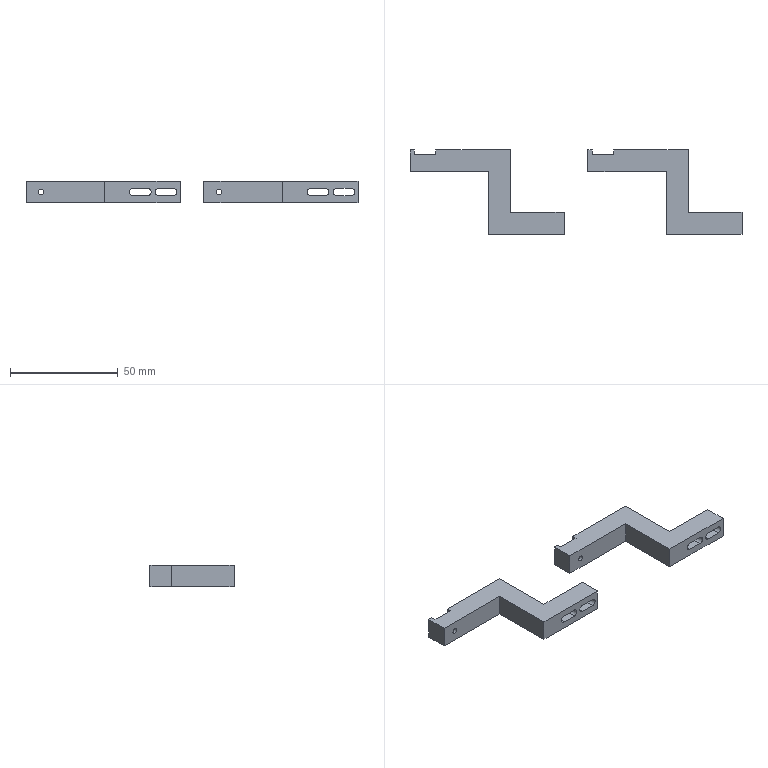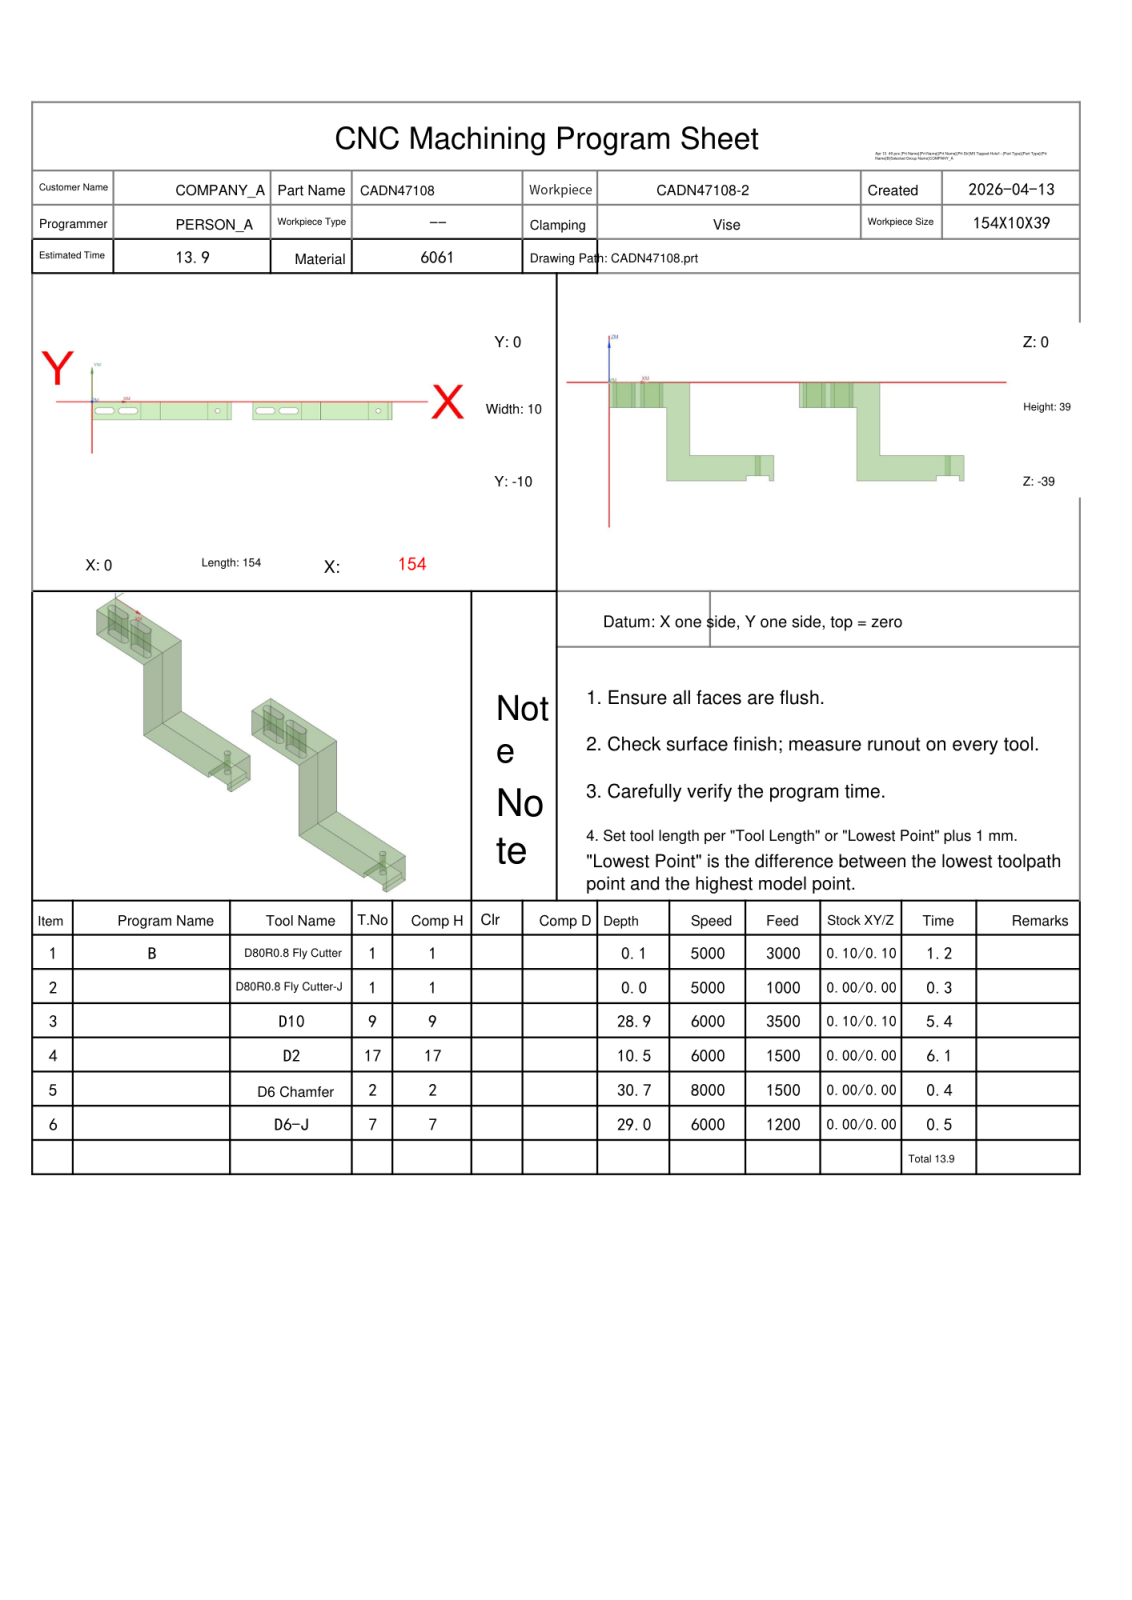NC program | NX | posted by the shop | part box 154 x 39 x 10 mm
Lines 2223 to 3149 of 5887:
N4 T17 M06
(D2  D=2. R=0. H=17 ce=0.10 di=0.10)
G00 G90 G54 X18.5 Y-4.4 M03 S6000
G43 H17 Z20.
M08
Z.5
G01 X15.2 Z.481 F1500.
G03 X14.6 Y-5. Z.475 I0.0 J-.6
X15.2 Y-5.6 Z.47 I.6 J0.0
G01 X21.8 Z.431
G03 X22.4 Y-5. Z.426 I0.0 J.6
X21.8 Y-4.4 Z.42 I-.6 J0.0
G01 X15.2 Z.382
G03 X14.6 Y-5. Z.376 I0.0 J-.6
X15.2 Y-5.6 Z.371 I.6 J0.0
G01 X21.8 Z.332
G03 X22.4 Y-5. Z.327 I0.0 J.6
X21.8 Y-4.4 Z.321 I-.6 J0.0
G01 X15.2 Z.283
G03 X14.6 Y-5. Z.277 I0.0 J-.6
X15.2 Y-5.6 Z.272 I.6 J0.0
G01 X21.8 Z.233
G03 X22.4 Y-5. Z.227 I0.0 J.6
X21.8 Y-4.4 Z.222 I-.6 J0.0
G01 X15.2 Z.183
G03 X14.6 Y-5. Z.178 I0.0 J-.6
X15.2 Y-5.6 Z.172 I.6 J0.0
G01 X21.8 Z.134
G03 X22.4 Y-5. Z.128 I0.0 J.6
X21.8 Y-4.4 Z.123 I-.6 J0.0
G01 X15.2 Z.084
G03 X14.6 Y-5. Z.079 I0.0 J-.6
X15.2 Y-5.6 Z.073 I.6 J0.0
G01 X21.8 Z.035
G03 X22.4 Y-5. Z.029 I0.0 J.6
X21.8 Y-4.4 Z.024 I-.6 J0.0
G01 X15.2 Z-.015
G03 X14.6 Y-5. Z-.02 I0.0 J-.6
X15.2 Y-5.6 Z-.026 I.6 J0.0
G01 X21.8 Z-.064
G03 X22.4 Y-5. Z-.07 I0.0 J.6
X21.8 Y-4.4 Z-.075 I-.6 J0.0
G01 X15.2 Z-.114
G03 X14.6 Y-5. Z-.119 I0.0 J-.6
X15.2 Y-5.6 Z-.125 I.6 J0.0
G01 X21.8 Z-.163
G03 X22.4 Y-5. Z-.169 I0.0 J.6
X21.8 Y-4.4 Z-.174 I-.6 J0.0
G01 X15.2 Z-.213
G03 X14.6 Y-5. Z-.218 I0.0 J-.6
X15.2 Y-5.6 Z-.224 I.6 J0.0
G01 X21.8 Z-.263
G03 X22.4 Y-5. Z-.268 I0.0 J.6
X21.8 Y-4.4 Z-.274 I-.6 J0.0
G01 X15.2 Z-.312
G03 X14.6 Y-5. Z-.318 I0.0 J-.6
X15.2 Y-5.6 Z-.323 I.6 J0.0
G01 X21.8 Z-.362
G03 X22.4 Y-5. Z-.367 I0.0 J.6
X21.8 Y-4.4 Z-.373 I-.6 J0.0
G01 X15.2 Z-.411
G03 X14.6 Y-5. Z-.417 I0.0 J-.6
X15.2 Y-5.6 Z-.422 I.6 J0.0
G01 X21.8 Z-.461
G03 X22.4 Y-5. Z-.466 I0.0 J.6
X21.8 Y-4.4 Z-.472 I-.6 J0.0
G01 X15.2 Z-.51
G03 X14.6 Y-5. Z-.516 I0.0 J-.6
X15.2 Y-5.6 Z-.521 I.6 J0.0
G01 X21.8 Z-.56
G03 X22.4 Y-5. Z-.565 I0.0 J.6
X21.8 Y-4.4 Z-.571 I-.6 J0.0
G01 X15.2 Z-.609
G03 X14.6 Y-5. Z-.615 I0.0 J-.6
X15.2 Y-5.6 Z-.62 I.6 J0.0
G01 X21.8 Z-.659
G03 X22.4 Y-5. Z-.664 I0.0 J.6
X21.8 Y-4.4 Z-.67 I-.6 J0.0
G01 X15.2 Z-.708
G03 X14.6 Y-5. Z-.714 I0.0 J-.6
X15.2 Y-5.6 Z-.719 I.6 J0.0
G01 X21.8 Z-.758
G03 X22.4 Y-5. Z-.764 I0.0 J.6
X21.8 Y-4.4 Z-.769 I-.6 J0.0
G01 X15.2 Z-.808
G03 X14.6 Y-5. Z-.813 I0.0 J-.6
X15.2 Y-5.6 Z-.819 I.6 J0.0
G01 X21.8 Z-.857
G03 X22.4 Y-5. Z-.863 I0.0 J.6
X21.8 Y-4.4 Z-.868 I-.6 J0.0
G01 X15.2 Z-.907
G03 X14.6 Y-5. Z-.912 I0.0 J-.6
X15.2 Y-5.6 Z-.918 I.6 J0.0
G01 X21.8 Z-.956
G03 X22.4 Y-5. Z-.962 I0.0 J.6
X21.8 Y-4.4 Z-.967 I-.6 J0.0
G01 X15.2 Z-1.006
G03 X14.6 Y-5. Z-1.011 I0.0 J-.6
X15.2 Y-5.6 Z-1.017 I.6 J0.0
G01 X21.8 Z-1.055
G03 X22.4 Y-5. Z-1.061 I0.0 J.6
X21.8 Y-4.4 Z-1.066 I-.6 J0.0
G01 X15.2 Z-1.105
G03 X14.6 Y-5. Z-1.11 I0.0 J-.6
X15.2 Y-5.6 Z-1.116 I.6 J0.0
G01 X21.8 Z-1.154
G03 X22.4 Y-5. Z-1.16 I0.0 J.6
X21.8 Y-4.4 Z-1.165 I-.6 J0.0
G01 X15.2 Z-1.204
G03 X14.6 Y-5. Z-1.209 I0.0 J-.6
X15.2 Y-5.6 Z-1.215 I.6 J0.0
G01 X21.8 Z-1.254
G03 X22.4 Y-5. Z-1.259 I0.0 J.6
X21.8 Y-4.4 Z-1.265 I-.6 J0.0
G01 X15.2 Z-1.303
G03 X14.6 Y-5. Z-1.309 I0.0 J-.6
X15.2 Y-5.6 Z-1.314 I.6 J0.0
G01 X21.8 Z-1.353
G03 X22.4 Y-5. Z-1.358 I0.0 J.6
X21.8 Y-4.4 Z-1.364 I-.6 J0.0
G01 X15.2 Z-1.402
G03 X14.6 Y-5. Z-1.408 I0.0 J-.6
X15.2 Y-5.6 Z-1.413 I.6 J0.0
G01 X21.8 Z-1.452
G03 X22.4 Y-5. Z-1.457 I0.0 J.6
X21.8 Y-4.4 Z-1.463 I-.6 J0.0
G01 X15.2 Z-1.501
G03 X14.6 Y-5. Z-1.507 I0.0 J-.6
X15.2 Y-5.6 Z-1.512 I.6 J0.0
G01 X21.8 Z-1.551
G03 X22.4 Y-5. Z-1.556 I0.0 J.6
X21.8 Y-4.4 Z-1.562 I-.6 J0.0
G01 X15.2 Z-1.6
G03 X14.6 Y-5. Z-1.606 I0.0 J-.6
X15.2 Y-5.6 Z-1.611 I.6 J0.0
G01 X21.8 Z-1.65
G03 X22.4 Y-5. Z-1.655 I0.0 J.6
X21.8 Y-4.4 Z-1.661 I-.6 J0.0
G01 X15.2 Z-1.699
G03 X14.6 Y-5. Z-1.705 I0.0 J-.6
X15.2 Y-5.6 Z-1.71 I.6 J0.0
G01 X21.8 Z-1.749
G03 X22.4 Y-5. Z-1.755 I0.0 J.6
X21.8 Y-4.4 Z-1.76 I-.6 J0.0
G01 X15.2 Z-1.799
G03 X14.6 Y-5. Z-1.804 I0.0 J-.6
X15.2 Y-5.6 Z-1.81 I.6 J0.0
G01 X21.8 Z-1.848
G03 X22.4 Y-5. Z-1.854 I0.0 J.6
X21.8 Y-4.4 Z-1.859 I-.6 J0.0
G01 X15.2 Z-1.898
G03 X14.6 Y-5. Z-1.903 I0.0 J-.6
X15.2 Y-5.6 Z-1.909 I.6 J0.0
G01 X21.8 Z-1.947
G03 X22.4 Y-5. Z-1.953 I0.0 J.6
X21.8 Y-4.4 Z-1.958 I-.6 J0.0
G01 X15.2 Z-1.997
G03 X14.6 Y-5. Z-2.002 I0.0 J-.6
X15.2 Y-5.6 Z-2.008 I.6 J0.0
G01 X21.8 Z-2.046
G03 X22.4 Y-5. Z-2.052 I0.0 J.6
X21.8 Y-4.4 Z-2.057 I-.6 J0.0
G01 X15.2 Z-2.096
G03 X14.6 Y-5. Z-2.101 I0.0 J-.6
X15.2 Y-5.6 Z-2.107 I.6 J0.0
G01 X21.8 Z-2.145
G03 X22.4 Y-5. Z-2.151 I0.0 J.6
X21.8 Y-4.4 Z-2.156 I-.6 J0.0
G01 X15.2 Z-2.195
G03 X14.6 Y-5. Z-2.2 I0.0 J-.6
X15.2 Y-5.6 Z-2.206 I.6 J0.0
G01 X21.8 Z-2.244
G03 X22.4 Y-5. Z-2.25 I0.0 J.6
X21.8 Y-4.4 Z-2.256 I-.6 J0.0
G01 X15.2 Z-2.294
G03 X14.6 Y-5. Z-2.3 I0.0 J-.6
X15.2 Y-5.6 Z-2.305 I.6 J0.0
G01 X21.8 Z-2.344
G03 X22.4 Y-5. Z-2.349 I0.0 J.6
X21.8 Y-4.4 Z-2.355 I-.6 J0.0
G01 X15.2 Z-2.393
G03 X14.6 Y-5. Z-2.399 I0.0 J-.6
X15.2 Y-5.6 Z-2.404 I.6 J0.0
G01 X21.8 Z-2.443
G03 X22.4 Y-5. Z-2.448 I0.0 J.6
X21.8 Y-4.4 Z-2.454 I-.6 J0.0
G01 X15.2 Z-2.492
G03 X14.6 Y-5. Z-2.498 I0.0 J-.6
X15.2 Y-5.6 Z-2.503 I.6 J0.0
G01 X21.8 Z-2.542
G03 X22.4 Y-5. Z-2.547 I0.0 J.6
X21.8 Y-4.4 Z-2.553 I-.6 J0.0
G01 X15.2 Z-2.591
G03 X14.6 Y-5. Z-2.597 I0.0 J-.6
X15.2 Y-5.6 Z-2.602 I.6 J0.0
G01 X21.8 Z-2.641
G03 X22.4 Y-5. Z-2.646 I0.0 J.6
X21.8 Y-4.4 Z-2.652 I-.6 J0.0
G01 X15.2 Z-2.69
G03 X14.6 Y-5. Z-2.696 I0.0 J-.6
X15.2 Y-5.6 Z-2.701 I.6 J0.0
G01 X21.8 Z-2.74
G03 X22.4 Y-5. Z-2.745 I0.0 J.6
X21.8 Y-4.4 Z-2.751 I-.6 J0.0
G01 X15.2 Z-2.79
G03 X14.6 Y-5. Z-2.795 I0.0 J-.6
X15.2 Y-5.6 Z-2.801 I.6 J0.0
G01 X21.8 Z-2.839
G03 X22.4 Y-5. Z-2.845 I0.0 J.6
X21.8 Y-4.4 Z-2.85 I-.6 J0.0
G01 X15.2 Z-2.889
G03 X14.6 Y-5. Z-2.894 I0.0 J-.6
X15.2 Y-5.6 Z-2.9 I.6 J0.0
G01 X21.8 Z-2.938
G03 X22.4 Y-5. Z-2.944 I0.0 J.6
X21.8 Y-4.4 Z-2.949 I-.6 J0.0
G01 X15.2 Z-2.988
G03 X14.6 Y-5. Z-2.993 I0.0 J-.6
X15.2 Y-5.6 Z-2.999 I.6 J0.0
G01 X21.8 Z-3.037
G03 X22.4 Y-5. Z-3.043 I0.0 J.6
X21.8 Y-4.4 Z-3.048 I-.6 J0.0
G01 X15.2 Z-3.087
G03 X14.6 Y-5. Z-3.092 I0.0 J-.6
X15.2 Y-5.6 Z-3.098 I.6 J0.0
G01 X21.8 Z-3.136
G03 X22.4 Y-5. Z-3.142 I0.0 J.6
X21.8 Y-4.4 Z-3.147 I-.6 J0.0
G01 X15.2 Z-3.186
G03 X14.6 Y-5. Z-3.191 I0.0 J-.6
X15.2 Y-5.6 Z-3.197 I.6 J0.0
G01 X21.8 Z-3.235
G03 X22.4 Y-5. Z-3.241 I0.0 J.6
X21.8 Y-4.4 Z-3.246 I-.6 J0.0
G01 X15.2 Z-3.285
G03 X14.6 Y-5. Z-3.291 I0.0 J-.6
X15.2 Y-5.6 Z-3.296 I.6 J0.0
G01 X21.8 Z-3.335
G03 X22.4 Y-5. Z-3.34 I0.0 J.6
X21.8 Y-4.4 Z-3.346 I-.6 J0.0
G01 X15.2 Z-3.384
G03 X14.6 Y-5. Z-3.39 I0.0 J-.6
X15.2 Y-5.6 Z-3.395 I.6 J0.0
G01 X21.8 Z-3.434
G03 X22.4 Y-5. Z-3.439 I0.0 J.6
X21.8 Y-4.4 Z-3.445 I-.6 J0.0
G01 X15.2 Z-3.483
G03 X14.6 Y-5. Z-3.489 I0.0 J-.6
X15.2 Y-5.6 Z-3.494 I.6 J0.0
G01 X21.8 Z-3.533
G03 X22.4 Y-5. Z-3.538 I0.0 J.6
X21.8 Y-4.4 Z-3.544 I-.6 J0.0
G01 X15.2 Z-3.582
G03 X14.6 Y-5. Z-3.588 I0.0 J-.6
X15.2 Y-5.6 Z-3.593 I.6 J0.0
G01 X21.8 Z-3.632
G03 X22.4 Y-5. Z-3.637 I0.0 J.6
X21.8 Y-4.4 Z-3.643 I-.6 J0.0
G01 X15.2 Z-3.681
G03 X14.6 Y-5. Z-3.687 I0.0 J-.6
X15.2 Y-5.6 Z-3.692 I.6 J0.0
G01 X21.8 Z-3.731
G03 X22.4 Y-5. Z-3.736 I0.0 J.6
X21.8 Y-4.4 Z-3.742 I-.6 J0.0
G01 X15.2 Z-3.781
G03 X14.6 Y-5. Z-3.786 I0.0 J-.6
X15.2 Y-5.6 Z-3.792 I.6 J0.0
G01 X21.8 Z-3.83
G03 X22.4 Y-5. Z-3.836 I0.0 J.6
X21.8 Y-4.4 Z-3.841 I-.6 J0.0
G01 X15.2 Z-3.88
G03 X14.6 Y-5. Z-3.885 I0.0 J-.6
X15.2 Y-5.6 Z-3.891 I.6 J0.0
G01 X21.8 Z-3.929
G03 X22.4 Y-5. Z-3.935 I0.0 J.6
X21.8 Y-4.4 Z-3.94 I-.6 J0.0
G01 X15.2 Z-3.979
G03 X14.6 Y-5. Z-3.984 I0.0 J-.6
X15.2 Y-5.6 Z-3.99 I.6 J0.0
G01 X21.8 Z-4.028
G03 X22.4 Y-5. Z-4.034 I0.0 J.6
X21.8 Y-4.4 Z-4.039 I-.6 J0.0
G01 X15.2 Z-4.078
G03 X14.6 Y-5. Z-4.083 I0.0 J-.6
X15.2 Y-5.6 Z-4.089 I.6 J0.0
G01 X21.8 Z-4.127
G03 X22.4 Y-5. Z-4.133 I0.0 J.6
X21.8 Y-4.4 Z-4.138 I-.6 J0.0
G01 X15.2 Z-4.177
G03 X14.6 Y-5. Z-4.182 I0.0 J-.6
X15.2 Y-5.6 Z-4.188 I.6 J0.0
G01 X21.8 Z-4.226
G03 X22.4 Y-5. Z-4.232 I0.0 J.6
X21.8 Y-4.4 Z-4.237 I-.6 J0.0
G01 X15.2 Z-4.276
G03 X14.6 Y-5. Z-4.282 I0.0 J-.6
X15.2 Y-5.6 Z-4.287 I.6 J0.0
G01 X21.8 Z-4.326
G03 X22.4 Y-5. Z-4.331 I0.0 J.6
X21.8 Y-4.4 Z-4.337 I-.6 J0.0
G01 X15.2 Z-4.375
G03 X14.6 Y-5. Z-4.381 I0.0 J-.6
X15.2 Y-5.6 Z-4.386 I.6 J0.0
G01 X21.8 Z-4.425
G03 X22.4 Y-5. Z-4.43 I0.0 J.6
X21.8 Y-4.4 Z-4.436 I-.6 J0.0
G01 X15.2 Z-4.474
G03 X14.6 Y-5. Z-4.48 I0.0 J-.6
X15.2 Y-5.6 Z-4.485 I.6 J0.0
G01 X21.8 Z-4.524
G03 X22.4 Y-5. Z-4.529 I0.0 J.6
X21.8 Y-4.4 Z-4.535 I-.6 J0.0
G01 X15.2 Z-4.573
G03 X14.6 Y-5. Z-4.579 I0.0 J-.6
X15.2 Y-5.6 Z-4.584 I.6 J0.0
G01 X21.8 Z-4.623
G03 X22.4 Y-5. Z-4.628 I0.0 J.6
X21.8 Y-4.4 Z-4.634 I-.6 J0.0
G01 X15.2 Z-4.672
G03 X14.6 Y-5. Z-4.678 I0.0 J-.6
X15.2 Y-5.6 Z-4.683 I.6 J0.0
G01 X21.8 Z-4.722
G03 X22.4 Y-5. Z-4.727 I0.0 J.6
X21.8 Y-4.4 Z-4.733 I-.6 J0.0
G01 X15.2 Z-4.772
G03 X14.6 Y-5. Z-4.777 I0.0 J-.6
X15.2 Y-5.6 Z-4.783 I.6 J0.0
G01 X21.8 Z-4.821
G03 X22.4 Y-5. Z-4.827 I0.0 J.6
X21.8 Y-4.4 Z-4.832 I-.6 J0.0
G01 X15.2 Z-4.871
G03 X14.6 Y-5. Z-4.876 I0.0 J-.6
X15.2 Y-5.6 Z-4.882 I.6 J0.0
G01 X21.8 Z-4.92
G03 X22.4 Y-5. Z-4.926 I0.0 J.6
X21.8 Y-4.4 Z-4.931 I-.6 J0.0
G01 X15.2 Z-4.97
G03 X14.6 Y-5. Z-4.975 I0.0 J-.6
X15.2 Y-5.6 Z-4.981 I.6 J0.0
G01 X21.8 Z-5.019
G03 X22.4 Y-5. Z-5.025 I0.0 J.6
X21.8 Y-4.4 Z-5.03 I-.6 J0.0
G01 X15.2 Z-5.069
G03 X14.6 Y-5. Z-5.074 I0.0 J-.6
X15.2 Y-5.6 Z-5.08 I.6 J0.0
G01 X21.8 Z-5.118
G03 X22.4 Y-5. Z-5.124 I0.0 J.6
X21.8 Y-4.4 Z-5.129 I-.6 J0.0
G01 X15.2 Z-5.168
G03 X14.6 Y-5. Z-5.173 I0.0 J-.6
X15.2 Y-5.6 Z-5.179 I.6 J0.0
G01 X21.8 Z-5.217
G03 X22.4 Y-5. Z-5.223 I0.0 J.6
X21.8 Y-4.4 Z-5.228 I-.6 J0.0
G01 X15.2 Z-5.267
G03 X14.6 Y-5. Z-5.273 I0.0 J-.6
X15.2 Y-5.6 Z-5.278 I.6 J0.0
G01 X21.8 Z-5.317
G03 X22.4 Y-5. Z-5.322 I0.0 J.6
X21.8 Y-4.4 Z-5.328 I-.6 J0.0
G01 X15.2 Z-5.366
G03 X14.6 Y-5. Z-5.372 I0.0 J-.6
X15.2 Y-5.6 Z-5.377 I.6 J0.0
G01 X21.8 Z-5.416
G03 X22.4 Y-5. Z-5.421 I0.0 J.6
X21.8 Y-4.4 Z-5.427 I-.6 J0.0
G01 X15.2 Z-5.465
G03 X14.6 Y-5. Z-5.471 I0.0 J-.6
X15.2 Y-5.6 Z-5.476 I.6 J0.0
G01 X21.8 Z-5.515
G03 X22.4 Y-5. Z-5.52 I0.0 J.6
X21.8 Y-4.4 Z-5.526 I-.6 J0.0
G01 X15.2 Z-5.564
G03 X14.6 Y-5. Z-5.57 I0.0 J-.6
X15.2 Y-5.6 Z-5.575 I.6 J0.0
G01 X21.8 Z-5.614
G03 X22.4 Y-5. Z-5.619 I0.0 J.6
X21.8 Y-4.4 Z-5.625 I-.6 J0.0
G01 X15.2 Z-5.663
G03 X14.6 Y-5. Z-5.669 I0.0 J-.6
X15.2 Y-5.6 Z-5.674 I.6 J0.0
G01 X21.8 Z-5.713
G03 X22.4 Y-5. Z-5.718 I0.0 J.6
X21.8 Y-4.4 Z-5.724 I-.6 J0.0
G01 X15.2 Z-5.763
G03 X14.6 Y-5. Z-5.768 I0.0 J-.6
X15.2 Y-5.6 Z-5.774 I.6 J0.0
G01 X21.8 Z-5.812
G03 X22.4 Y-5. Z-5.818 I0.0 J.6
X21.8 Y-4.4 Z-5.823 I-.6 J0.0
G01 X15.2 Z-5.862
G03 X14.6 Y-5. Z-5.867 I0.0 J-.6
X15.2 Y-5.6 Z-5.873 I.6 J0.0
G01 X21.8 Z-5.911
G03 X22.4 Y-5. Z-5.917 I0.0 J.6
X21.8 Y-4.4 Z-5.922 I-.6 J0.0
G01 X15.2 Z-5.961
G03 X14.6 Y-5. Z-5.966 I0.0 J-.6
X15.2 Y-5.6 Z-5.972 I.6 J0.0
G01 X21.8 Z-6.01
G03 X22.4 Y-5. Z-6.016 I0.0 J.6
X21.8 Y-4.4 Z-6.021 I-.6 J0.0
G01 X15.2 Z-6.06
G03 X14.6 Y-5. Z-6.065 I0.0 J-.6
X15.2 Y-5.6 Z-6.071 I.6 J0.0
G01 X21.8 Z-6.109
G03 X22.4 Y-5. Z-6.115 I0.0 J.6
X21.8 Y-4.4 Z-6.12 I-.6 J0.0
G01 X15.2 Z-6.159
G03 X14.6 Y-5. Z-6.164 I0.0 J-.6
X15.2 Y-5.6 Z-6.17 I.6 J0.0
G01 X21.8 Z-6.208
G03 X22.4 Y-5. Z-6.214 I0.0 J.6
X21.8 Y-4.4 Z-6.219 I-.6 J0.0
G01 X15.2 Z-6.258
G03 X14.6 Y-5. Z-6.264 I0.0 J-.6
X15.2 Y-5.6 Z-6.269 I.6 J0.0
G01 X21.8 Z-6.308
G03 X22.4 Y-5. Z-6.313 I0.0 J.6
X21.8 Y-4.4 Z-6.319 I-.6 J0.0
G01 X15.2 Z-6.357
G03 X14.6 Y-5. Z-6.363 I0.0 J-.6
X15.2 Y-5.6 Z-6.368 I.6 J0.0
G01 X21.8 Z-6.407
G03 X22.4 Y-5. Z-6.412 I0.0 J.6
X21.8 Y-4.4 Z-6.418 I-.6 J0.0
G01 X15.2 Z-6.456
G03 X14.6 Y-5. Z-6.462 I0.0 J-.6
X15.2 Y-5.6 Z-6.467 I.6 J0.0
G01 X21.8 Z-6.506
G03 X22.4 Y-5. Z-6.511 I0.0 J.6
X21.8 Y-4.4 Z-6.517 I-.6 J0.0
G01 X15.2 Z-6.555
G03 X14.6 Y-5. Z-6.561 I0.0 J-.6
X15.2 Y-5.6 Z-6.566 I.6 J0.0
G01 X21.8 Z-6.605
G03 X22.4 Y-5. Z-6.61 I0.0 J.6
X21.8 Y-4.4 Z-6.616 I-.6 J0.0
G01 X15.2 Z-6.654
G03 X14.6 Y-5. Z-6.66 I0.0 J-.6
X15.2 Y-5.6 Z-6.665 I.6 J0.0
G01 X21.8 Z-6.704
G03 X22.4 Y-5. Z-6.709 I0.0 J.6
X21.8 Y-4.4 Z-6.715 I-.6 J0.0
G01 X15.2 Z-6.754
G03 X14.6 Y-5. Z-6.759 I0.0 J-.6
X15.2 Y-5.6 Z-6.765 I.6 J0.0
G01 X21.8 Z-6.803
G03 X22.4 Y-5. Z-6.809 I0.0 J.6
X21.8 Y-4.4 Z-6.814 I-.6 J0.0
G01 X15.2 Z-6.853
G03 X14.6 Y-5. Z-6.858 I0.0 J-.6
X15.2 Y-5.6 Z-6.864 I.6 J0.0
G01 X21.8 Z-6.902
G03 X22.4 Y-5. Z-6.908 I0.0 J.6
X21.8 Y-4.4 Z-6.913 I-.6 J0.0
G01 X15.2 Z-6.952
G03 X14.6 Y-5. Z-6.957 I0.0 J-.6
X15.2 Y-5.6 Z-6.963 I.6 J0.0
G01 X21.8 Z-7.001
G03 X22.4 Y-5. Z-7.007 I0.0 J.6
X21.8 Y-4.4 Z-7.012 I-.6 J0.0
G01 X15.2 Z-7.051
G03 X14.6 Y-5. Z-7.056 I0.0 J-.6
X15.2 Y-5.6 Z-7.062 I.6 J0.0
G01 X21.8 Z-7.1
G03 X22.4 Y-5. Z-7.106 I0.0 J.6
X21.8 Y-4.4 Z-7.111 I-.6 J0.0
G01 X15.2 Z-7.15
G03 X14.6 Y-5. Z-7.155 I0.0 J-.6
X15.2 Y-5.6 Z-7.161 I.6 J0.0
G01 X21.8 Z-7.199
G03 X22.4 Y-5. Z-7.205 I0.0 J.6
X21.8 Y-4.4 Z-7.21 I-.6 J0.0
G01 X15.2 Z-7.249
G03 X14.6 Y-5. Z-7.255 I0.0 J-.6
X15.2 Y-5.6 Z-7.26 I.6 J0.0
G01 X21.8 Z-7.299
G03 X22.4 Y-5. Z-7.304 I0.0 J.6
X21.8 Y-4.4 Z-7.31 I-.6 J0.0
G01 X15.2 Z-7.348
G03 X14.6 Y-5. Z-7.354 I0.0 J-.6
X15.2 Y-5.6 Z-7.359 I.6 J0.0
G01 X21.8 Z-7.398
G03 X22.4 Y-5. Z-7.403 I0.0 J.6
X21.8 Y-4.4 Z-7.409 I-.6 J0.0
G01 X15.2 Z-7.447
G03 X14.6 Y-5. Z-7.453 I0.0 J-.6
X15.2 Y-5.6 Z-7.458 I.6 J0.0
G01 X21.8 Z-7.497
G03 X22.4 Y-5. Z-7.502 I0.0 J.6
X21.8 Y-4.4 Z-7.508 I-.6 J0.0
G01 X15.2 Z-7.546
G03 X14.6 Y-5. Z-7.552 I0.0 J-.6
X15.2 Y-5.6 Z-7.557 I.6 J0.0
G01 X21.8 Z-7.596
G03 X22.4 Y-5. Z-7.601 I0.0 J.6
X21.8 Y-4.4 Z-7.607 I-.6 J0.0
G01 X15.2 Z-7.645
G03 X14.6 Y-5. Z-7.651 I0.0 J-.6
X15.2 Y-5.6 Z-7.656 I.6 J0.0
G01 X21.8 Z-7.695
G03 X22.4 Y-5. Z-7.7 I0.0 J.6
X21.8 Y-4.4 Z-7.706 I-.6 J0.0
G01 X15.2 Z-7.744
G03 X14.6 Y-5. Z-7.75 I0.0 J-.6
X15.2 Y-5.6 Z-7.756 I.6 J0.0
G01 X21.8 Z-7.794
G03 X22.4 Y-5. Z-7.8 I0.0 J.6
X21.8 Y-4.4 Z-7.805 I-.6 J0.0
G01 X15.2 Z-7.844
G03 X14.6 Y-5. Z-7.849 I0.0 J-.6
X15.2 Y-5.6 Z-7.855 I.6 J0.0
G01 X21.8 Z-7.893
G03 X22.4 Y-5. Z-7.899 I0.0 J.6
X21.8 Y-4.4 Z-7.904 I-.6 J0.0
G01 X15.2 Z-7.943
G03 X14.6 Y-5. Z-7.948 I0.0 J-.6
X15.2 Y-5.6 Z-7.954 I.6 J0.0
G01 X21.8 Z-7.992
G03 X22.4 Y-5. Z-7.998 I0.0 J.6
X21.8 Y-4.4 Z-8.003 I-.6 J0.0
G01 X15.2 Z-8.042
G03 X14.6 Y-5. Z-8.047 I0.0 J-.6
X15.2 Y-5.6 Z-8.053 I.6 J0.0
G01 X21.8 Z-8.091
G03 X22.4 Y-5. Z-8.097 I0.0 J.6
X21.8 Y-4.4 Z-8.102 I-.6 J0.0
G01 X15.2 Z-8.141
G03 X14.6 Y-5. Z-8.146 I0.0 J-.6
X15.2 Y-5.6 Z-8.152 I.6 J0.0
G01 X21.8 Z-8.19
G03 X22.4 Y-5. Z-8.196 I0.0 J.6
X21.8 Y-4.4 Z-8.201 I-.6 J0.0
G01 X15.2 Z-8.24
G03 X14.6 Y-5. Z-8.245 I0.0 J-.6
X15.2 Y-5.6 Z-8.251 I.6 J0.0
G01 X21.8 Z-8.29
G03 X22.4 Y-5. Z-8.295 I0.0 J.6
X21.8 Y-4.4 Z-8.301 I-.6 J0.0
G01 X15.2 Z-8.339
G03 X14.6 Y-5. Z-8.345 I0.0 J-.6
X15.2 Y-5.6 Z-8.35 I.6 J0.0
G01 X21.8 Z-8.389
G03 X22.4 Y-5. Z-8.394 I0.0 J.6
X21.8 Y-4.4 Z-8.4 I-.6 J0.0
G01 X15.2 Z-8.438
G03 X14.6 Y-5. Z-8.444 I0.0 J-.6
X15.2 Y-5.6 Z-8.449 I.6 J0.0
G01 X21.8 Z-8.488
G03 X22.4 Y-5. Z-8.493 I0.0 J.6
X21.8 Y-4.4 Z-8.499 I-.6 J0.0
G01 X15.2 Z-8.537
G03 X14.6 Y-5. Z-8.543 I0.0 J-.6
X15.2 Y-5.6 Z-8.548 I.6 J0.0
G01 X21.8 Z-8.587
G03 X22.4 Y-5. Z-8.592 I0.0 J.6
X21.8 Y-4.4 Z-8.598 I-.6 J0.0
G01 X15.2 Z-8.636
G03 X14.6 Y-5. Z-8.642 I0.0 J-.6
X15.2 Y-5.6 Z-8.647 I.6 J0.0
G01 X21.8 Z-8.686
G03 X22.4 Y-5. Z-8.691 I0.0 J.6
X21.8 Y-4.4 Z-8.697 I-.6 J0.0
G01 X15.2 Z-8.735
G03 X14.6 Y-5. Z-8.741 I0.0 J-.6
X15.2 Y-5.6 Z-8.746 I.6 J0.0
G01 X21.8 Z-8.785
G03 X22.4 Y-5. Z-8.791 I0.0 J.6
X21.8 Y-4.4 Z-8.796 I-.6 J0.0
G01 X15.2 Z-8.835
G03 X14.6 Y-5. Z-8.84 I0.0 J-.6
X15.2 Y-5.6 Z-8.846 I.6 J0.0
G01 X21.8 Z-8.884
G03 X22.4 Y-5. Z-8.89 I0.0 J.6
X21.8 Y-4.4 Z-8.895 I-.6 J0.0
G01 X15.2 Z-8.934
G03 X14.6 Y-5. Z-8.939 I0.0 J-.6
X15.2 Y-5.6 Z-8.945 I.6 J0.0
G01 X21.8 Z-8.983
G03 X22.4 Y-5. Z-8.989 I0.0 J.6
X21.8 Y-4.4 Z-8.994 I-.6 J0.0
G01 X15.2 Z-9.033
G03 X14.6 Y-5. Z-9.038 I0.0 J-.6
X15.2 Y-5.6 Z-9.044 I.6 J0.0
G01 X21.8 Z-9.082
G03 X22.4 Y-5. Z-9.088 I0.0 J.6
X21.8 Y-4.4 Z-9.093 I-.6 J0.0
G01 X15.2 Z-9.132
G03 X14.6 Y-5. Z-9.137 I0.0 J-.6
X15.2 Y-5.6 Z-9.143 I.6 J0.0
G01 X21.8 Z-9.181
G03 X22.4 Y-5. Z-9.187 I0.0 J.6
X21.8 Y-4.4 Z-9.192 I-.6 J0.0
G01 X15.2 Z-9.231
G03 X14.6 Y-5. Z-9.236 I0.0 J-.6
X15.2 Y-5.6 Z-9.242 I.6 J0.0
G01 X21.8 Z-9.281
G03 X22.4 Y-5. Z-9.286 I0.0 J.6
X21.8 Y-4.4 Z-9.292 I-.6 J0.0
G01 X15.2 Z-9.33
G03 X14.6 Y-5. Z-9.336 I0.0 J-.6
X15.2 Y-5.6 Z-9.341 I.6 J0.0
G01 X21.8 Z-9.38
G03 X22.4 Y-5. Z-9.385 I0.0 J.6
X21.8 Y-4.4 Z-9.391 I-.6 J0.0
G01 X15.2 Z-9.429
G03 X14.6 Y-5. Z-9.435 I0.0 J-.6
X15.2 Y-5.6 Z-9.44 I.6 J0.0
G01 X21.8 Z-9.479
G03 X22.4 Y-5. Z-9.484 I0.0 J.6
X21.8 Y-4.4 Z-9.49 I-.6 J0.0
G01 X15.2 Z-9.528
G03 X14.6 Y-5. Z-9.534 I0.0 J-.6
X15.2 Y-5.6 Z-9.539 I.6 J0.0
G01 X21.8 Z-9.578
G03 X22.4 Y-5. Z-9.583 I0.0 J.6
X21.8 Y-4.4 Z-9.589 I-.6 J0.0
G01 X15.2 Z-9.627
G03 X14.6 Y-5. Z-9.633 I0.0 J-.6
X15.2 Y-5.6 Z-9.638 I.6 J0.0
G01 X21.8 Z-9.677
G03 X22.4 Y-5. Z-9.682 I0.0 J.6
X21.8 Y-4.4 Z-9.688 I-.6 J0.0
G01 X15.2 Z-9.726
G03 X14.6 Y-5. Z-9.732 I0.0 J-.6
X15.2 Y-5.6 Z-9.737 I.6 J0.0
G01 X21.8 Z-9.776
G03 X22.4 Y-5. Z-9.782 I0.0 J.6
X21.8 Y-4.4 Z-9.787 I-.6 J0.0
G01 X15.2 Z-9.826
G03 X14.6 Y-5. Z-9.831 I0.0 J-.6
X15.2 Y-5.6 Z-9.837 I.6 J0.0
G01 X21.8 Z-9.875
G03 X22.4 Y-5. Z-9.881 I0.0 J.6
X21.8 Y-4.4 Z-9.886 I-.6 J0.0
G01 X15.2 Z-9.925
G03 X14.6 Y-5. Z-9.93 I0.0 J-.6
X15.2 Y-5.6 Z-9.936 I.6 J0.0
G01 X21.8 Z-9.974
G03 X22.4 Y-5. Z-9.98 I0.0 J.6
X21.8 Y-4.4 Z-9.985 I-.6 J0.0
G01 X15.2 Z-10.024
G03 X14.6 Y-5. Z-10.029 I0.0 J-.6
X15.2 Y-5.6 Z-10.035 I.6 J0.0
G01 X21.8 Z-10.073
G03 X22.4 Y-5. Z-10.079 I0.0 J.6
X21.8 Y-4.4 Z-10.084 I-.6 J0.0
G01 X15.2 Z-10.123
G03 X14.6 Y-5. Z-10.128 I0.0 J-.6
X15.2 Y-5.6 Z-10.134 I.6 J0.0
G01 X21.8 Z-10.172
G03 X22.4 Y-5. Z-10.178 I0.0 J.6
X21.8 Y-4.4 Z-10.183 I-.6 J0.0
G01 X15.2 Z-10.222
G03 X14.6 Y-5. Z-10.227 I0.0 J-.6
X15.2 Y-5.6 Z-10.233 I.6 J0.0
G01 X21.8 Z-10.272
G03 X22.4 Y-5. Z-10.277 I0.0 J.6
X21.8 Y-4.4 Z-10.283 I-.6 J0.0
G01 X15.2 Z-10.321
G03 X14.6 Y-5. Z-10.327 I0.0 J-.6
X15.2 Y-5.6 Z-10.332 I.6 J0.0
G01 X21.8 Z-10.371
G03 X22.4 Y-5. Z-10.376 I0.0 J.6
X21.8 Y-4.4 Z-10.382 I-.6 J0.0
G01 X15.2 Z-10.42
G03 X14.6 Y-5. Z-10.426 I0.0 J-.6
X15.2 Y-5.6 Z-10.431 I.6 J0.0
G01 X21.8 Z-10.47
G03 X22.4 Y-5. Z-10.475 I0.0 J.6
X21.8 Y-4.4 Z-10.481 I-.6 J0.0
G01 X18.5 Z-10.5
X15.2
G03 X14.6 Y-5. I0.0 J-.6
X15.2 Y-5.6 I.6 J0.0
G01 X21.8
G03 X22.4 Y-5. I0.0 J.6
X21.8 Y-4.4 I-.6 J0.0
G01 X18.5
X18.
Z-9.5
G00 Z20.
X6.5 Y-5.6
Z.5
G01 X9.8 Z.481
G03 X10.4 Y-5. Z.475 I0.0 J.6
X9.8 Y-4.4 Z.47 I-.6 J0.0
G01 X3.2 Z.431
G03 X2.6 Y-5. Z.426 I0.0 J-.6
X3.2 Y-5.6 Z.42 I.6 J0.0
G01 X9.8 Z.382
G03 X10.4 Y-5. Z.376 I0.0 J.6
X9.8 Y-4.4 Z.371 I-.6 J0.0
G01 X3.2 Z.332
G03 X2.6 Y-5. Z.327 I0.0 J-.6
X3.2 Y-5.6 Z.321 I.6 J0.0
G01 X9.8 Z.283
G03 X10.4 Y-5. Z.277 I0.0 J.6
X9.8 Y-4.4 Z.272 I-.6 J0.0
G01 X3.2 Z.233
G03 X2.6 Y-5. Z.227 I0.0 J-.6
X3.2 Y-5.6 Z.222 I.6 J0.0
G01 X9.8 Z.183
G03 X10.4 Y-5. Z.178 I0.0 J.6
X9.8 Y-4.4 Z.172 I-.6 J0.0
G01 X3.2 Z.134
G03 X2.6 Y-5. Z.128 I0.0 J-.6
X3.2 Y-5.6 Z.123 I.6 J0.0
G01 X9.8 Z.084
G03 X10.4 Y-5. Z.079 I0.0 J.6
X9.8 Y-4.4 Z.073 I-.6 J0.0
G01 X3.2 Z.035
G03 X2.6 Y-5. Z.029 I0.0 J-.6
X3.2 Y-5.6 Z.024 I.6 J0.0
G01 X9.8 Z-.015
G03 X10.4 Y-5. Z-.02 I0.0 J.6
X9.8 Y-4.4 Z-.026 I-.6 J0.0
G01 X3.2 Z-.064
G03 X2.6 Y-5. Z-.07 I0.0 J-.6
X3.2 Y-5.6 Z-.075 I.6 J0.0
G01 X9.8 Z-.114
G03 X10.4 Y-5. Z-.119 I0.0 J.6
X9.8 Y-4.4 Z-.125 I-.6 J0.0
G01 X3.2 Z-.163
G03 X2.6 Y-5. Z-.169 I0.0 J-.6
X3.2 Y-5.6 Z-.174 I.6 J0.0
G01 X9.8 Z-.213
G03 X10.4 Y-5. Z-.218 I0.0 J.6
X9.8 Y-4.4 Z-.224 I-.6 J0.0
G01 X3.2 Z-.263
G03 X2.6 Y-5. Z-.268 I0.0 J-.6
X3.2 Y-5.6 Z-.274 I.6 J0.0
G01 X9.8 Z-.312
G03 X10.4 Y-5. Z-.318 I0.0 J.6
X9.8 Y-4.4 Z-.323 I-.6 J0.0
G01 X3.2 Z-.362
G03 X2.6 Y-5. Z-.367 I0.0 J-.6
X3.2 Y-5.6 Z-.373 I.6 J0.0
G01 X9.8 Z-.411
G03 X10.4 Y-5. Z-.417 I0.0 J.6
X9.8 Y-4.4 Z-.422 I-.6 J0.0
G01 X3.2 Z-.461
G03 X2.6 Y-5. Z-.466 I0.0 J-.6
X3.2 Y-5.6 Z-.472 I.6 J0.0
G01 X9.8 Z-.51
G03 X10.4 Y-5. Z-.516 I0.0 J.6
X9.8 Y-4.4 Z-.521 I-.6 J0.0
G01 X3.2 Z-.56
G03 X2.6 Y-5. Z-.565 I0.0 J-.6
X3.2 Y-5.6 Z-.571 I.6 J0.0
G01 X9.8 Z-.609
G03 X10.4 Y-5. Z-.615 I0.0 J.6
X9.8 Y-4.4 Z-.62 I-.6 J0.0
G01 X3.2 Z-.659
G03 X2.6 Y-5. Z-.664 I0.0 J-.6
X3.2 Y-5.6 Z-.67 I.6 J0.0
G01 X9.8 Z-.708
G03 X10.4 Y-5. Z-.714 I0.0 J.6
X9.8 Y-4.4 Z-.719 I-.6 J0.0
G01 X3.2 Z-.758
G03 X2.6 Y-5. Z-.764 I0.0 J-.6
X3.2 Y-5.6 Z-.769 I.6 J0.0
G01 X9.8 Z-.808
G03 X10.4 Y-5. Z-.813 I0.0 J.6
X9.8 Y-4.4 Z-.819 I-.6 J0.0
G01 X3.2 Z-.857
G03 X2.6 Y-5. Z-.863 I0.0 J-.6
X3.2 Y-5.6 Z-.868 I.6 J0.0
G01 X9.8 Z-.907
G03 X10.4 Y-5. Z-.912 I0.0 J.6
X9.8 Y-4.4 Z-.918 I-.6 J0.0
G01 X3.2 Z-.956
G03 X2.6 Y-5. Z-.962 I0.0 J-.6
X3.2 Y-5.6 Z-.967 I.6 J0.0
G01 X9.8 Z-1.006
G03 X10.4 Y-5. Z-1.011 I0.0 J.6
X9.8 Y-4.4 Z-1.017 I-.6 J0.0
G01 X3.2 Z-1.055
G03 X2.6 Y-5. Z-1.061 I0.0 J-.6
X3.2 Y-5.6 Z-1.066 I.6 J0.0
G01 X9.8 Z-1.105
G03 X10.4 Y-5. Z-1.11 I0.0 J.6
X9.8 Y-4.4 Z-1.116 I-.6 J0.0
G01 X3.2 Z-1.154
G03 X2.6 Y-5. Z-1.16 I0.0 J-.6
X3.2 Y-5.6 Z-1.165 I.6 J0.0
G01 X9.8 Z-1.204
G03 X10.4 Y-5. Z-1.209 I0.0 J.6
X9.8 Y-4.4 Z-1.215 I-.6 J0.0
G01 X3.2 Z-1.254
G03 X2.6 Y-5. Z-1.259 I0.0 J-.6
X3.2 Y-5.6 Z-1.265 I.6 J0.0
G01 X9.8 Z-1.303
G03 X10.4 Y-5. Z-1.309 I0.0 J.6
X9.8 Y-4.4 Z-1.314 I-.6 J0.0
G01 X3.2 Z-1.353
G03 X2.6 Y-5. Z-1.358 I0.0 J-.6
X3.2 Y-5.6 Z-1.364 I.6 J0.0
G01 X9.8 Z-1.402
G03 X10.4 Y-5. Z-1.408 I0.0 J.6
X9.8 Y-4.4 Z-1.413 I-.6 J0.0
G01 X3.2 Z-1.452
G03 X2.6 Y-5. Z-1.457 I0.0 J-.6
X3.2 Y-5.6 Z-1.463 I.6 J0.0
G01 X9.8 Z-1.501
G03 X10.4 Y-5. Z-1.507 I0.0 J.6
X9.8 Y-4.4 Z-1.512 I-.6 J0.0
G01 X3.2 Z-1.551
G03 X2.6 Y-5. Z-1.556 I0.0 J-.6
X3.2 Y-5.6 Z-1.562 I.6 J0.0
G01 X9.8 Z-1.6
G03 X10.4 Y-5. Z-1.606 I0.0 J.6
X9.8 Y-4.4 Z-1.611 I-.6 J0.0
G01 X3.2 Z-1.65
G03 X2.6 Y-5. Z-1.655 I0.0 J-.6
X3.2 Y-5.6 Z-1.661 I.6 J0.0
G01 X9.8 Z-1.699
G03 X10.4 Y-5. Z-1.705 I0.0 J.6
X9.8 Y-4.4 Z-1.71 I-.6 J0.0
G01 X3.2 Z-1.749
G03 X2.6 Y-5. Z-1.755 I0.0 J-.6
X3.2 Y-5.6 Z-1.76 I.6 J0.0
G01 X9.8 Z-1.799
G03 X10.4 Y-5. Z-1.804 I0.0 J.6
X9.8 Y-4.4 Z-1.81 I-.6 J0.0
G01 X3.2 Z-1.848
G03 X2.6 Y-5. Z-1.854 I0.0 J-.6
X3.2 Y-5.6 Z-1.859 I.6 J0.0
G01 X9.8 Z-1.898
G03 X10.4 Y-5. Z-1.903 I0.0 J.6
X9.8 Y-4.4 Z-1.909 I-.6 J0.0
G01 X3.2 Z-1.947
G03 X2.6 Y-5. Z-1.953 I0.0 J-.6
X3.2 Y-5.6 Z-1.958 I.6 J0.0
G01 X9.8 Z-1.997
G03 X10.4 Y-5. Z-2.002 I0.0 J.6
X9.8 Y-4.4 Z-2.008 I-.6 J0.0
G01 X3.2 Z-2.046
G03 X2.6 Y-5. Z-2.052 I0.0 J-.6
X3.2 Y-5.6 Z-2.057 I.6 J0.0
G01 X9.8 Z-2.096
G03 X10.4 Y-5. Z-2.101 I0.0 J.6
X9.8 Y-4.4 Z-2.107 I-.6 J0.0
G01 X3.2 Z-2.145
G03 X2.6 Y-5. Z-2.151 I0.0 J-.6
X3.2 Y-5.6 Z-2.156 I.6 J0.0
G01 X9.8 Z-2.195
G03 X10.4 Y-5. Z-2.2 I0.0 J.6
X9.8 Y-4.4 Z-2.206 I-.6 J0.0
G01 X3.2 Z-2.244
G03 X2.6 Y-5. Z-2.25 I0.0 J-.6
X3.2 Y-5.6 Z-2.256 I.6 J0.0
G01 X9.8 Z-2.294
G03 X10.4 Y-5. Z-2.3 I0.0 J.6
X9.8 Y-4.4 Z-2.305 I-.6 J0.0
G01 X3.2 Z-2.344
G03 X2.6 Y-5. Z-2.349 I0.0 J-.6
X3.2 Y-5.6 Z-2.355 I.6 J0.0
G01 X9.8 Z-2.393
G03 X10.4 Y-5. Z-2.399 I0.0 J.6
X9.8 Y-4.4 Z-2.404 I-.6 J0.0
G01 X3.2 Z-2.443
G03 X2.6 Y-5. Z-2.448 I0.0 J-.6
X3.2 Y-5.6 Z-2.454 I.6 J0.0
G01 X9.8 Z-2.492
G03 X10.4 Y-5. Z-2.498 I0.0 J.6
X9.8 Y-4.4 Z-2.503 I-.6 J0.0
G01 X3.2 Z-2.542
G03 X2.6 Y-5. Z-2.547 I0.0 J-.6
X3.2 Y-5.6 Z-2.553 I.6 J0.0
G01 X9.8 Z-2.591
G03 X10.4 Y-5. Z-2.597 I0.0 J.6
X9.8 Y-4.4 Z-2.602 I-.6 J0.0
G01 X3.2 Z-2.641
G03 X2.6 Y-5. Z-2.646 I0.0 J-.6
X3.2 Y-5.6 Z-2.652 I.6 J0.0
G01 X9.8 Z-2.69
G03 X10.4 Y-5. Z-2.696 I0.0 J.6
X9.8 Y-4.4 Z-2.701 I-.6 J0.0
G01 X3.2 Z-2.74
G03 X2.6 Y-5. Z-2.745 I0.0 J-.6
X3.2 Y-5.6 Z-2.751 I.6 J0.0
G01 X9.8 Z-2.79
G03 X10.4 Y-5. Z-2.795 I0.0 J.6
X9.8 Y-4.4 Z-2.801 I-.6 J0.0
G01 X3.2 Z-2.839
G03 X2.6 Y-5. Z-2.845 I0.0 J-.6
X3.2 Y-5.6 Z-2.85 I.6 J0.0
G01 X9.8 Z-2.889
G03 X10.4 Y-5. Z-2.894 I0.0 J.6
X9.8 Y-4.4 Z-2.9 I-.6 J0.0
G01 X3.2 Z-2.938
G03 X2.6 Y-5. Z-2.944 I0.0 J-.6
X3.2 Y-5.6 Z-2.949 I.6 J0.0
G01 X9.8 Z-2.988
G03 X10.4 Y-5. Z-2.993 I0.0 J.6
X9.8 Y-4.4 Z-2.999 I-.6 J0.0
G01 X3.2 Z-3.037
G03 X2.6 Y-5. Z-3.043 I0.0 J-.6
X3.2 Y-5.6 Z-3.048 I.6 J0.0
G01 X9.8 Z-3.087
G03 X10.4 Y-5. Z-3.092 I0.0 J.6
X9.8 Y-4.4 Z-3.098 I-.6 J0.0
G01 X3.2 Z-3.136
G03 X2.6 Y-5. Z-3.142 I0.0 J-.6
X3.2 Y-5.6 Z-3.147 I.6 J0.0
G01 X9.8 Z-3.186
G03 X10.4 Y-5. Z-3.191 I0.0 J.6
X9.8 Y-4.4 Z-3.197 I-.6 J0.0
G01 X3.2 Z-3.235
G03 X2.6 Y-5. Z-3.241 I0.0 J-.6
X3.2 Y-5.6 Z-3.246 I.6 J0.0
G01 X9.8 Z-3.285
G03 X10.4 Y-5. Z-3.291 I0.0 J.6
X9.8 Y-4.4 Z-3.296 I-.6 J0.0
G01 X3.2 Z-3.335
G03 X2.6 Y-5. Z-3.34 I0.0 J-.6
X3.2 Y-5.6 Z-3.346 I.6 J0.0
G01 X9.8 Z-3.384
G03 X10.4 Y-5. Z-3.39 I0.0 J.6
X9.8 Y-4.4 Z-3.395 I-.6 J0.0
G01 X3.2 Z-3.434
G03 X2.6 Y-5. Z-3.439 I0.0 J-.6
X3.2 Y-5.6 Z-3.445 I.6 J0.0
G01 X9.8 Z-3.483
G03 X10.4 Y-5. Z-3.489 I0.0 J.6